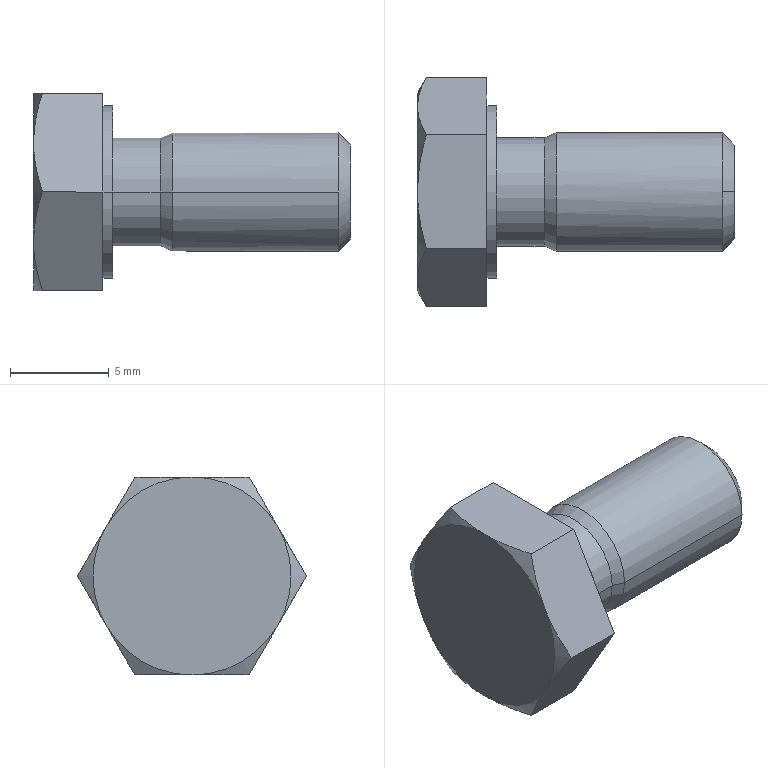Part | SolidWorks | features BaseBody 1 | 1 solid | 26 faces | box 16 x 11.547 x 10 mm | volume 654.588 mm3 | cone 10 | plane 10 | cylinder 6 | commonest cylinder face diameters 5.459 x2 6 x2 8.7 x2
STEP:
#1=CARTESIAN_POINT('',(3.,3.,0.));
#2=VERTEX_POINT('',#1);
#3=CARTESIAN_POINT('',(3.,-3.,0.));
#4=VERTEX_POINT('',#3);
#5=CARTESIAN_POINT('',(3.,0.,0.));
#6=DIRECTION('',(1.,0.,0.));
#7=DIRECTION('',(0.,1.,0.));
#8=AXIS2_PLACEMENT_3D('',#5,#6,#7);
#9=CIRCLE('',#8,3.);
#10=EDGE_CURVE('',#2,#4,#9,.T.);
#11=ORIENTED_EDGE('',*,*,#10,.T.);
#12=CARTESIAN_POINT('',(11.386,-3.,0.));
#13=VERTEX_POINT('',#12);
#14=CARTESIAN_POINT('',(7.5,-3.,0.));
#15=DIRECTION('',(1.,0.,0.));
#16=VECTOR('',#15,1000.);
#17=LINE('',#14,#16);
#18=EDGE_CURVE('',#4,#13,#17,.T.);
#19=ORIENTED_EDGE('',*,*,#18,.T.);
#20=CARTESIAN_POINT('',(11.386,0.,3.));
#21=VERTEX_POINT('',#20);
#22=CARTESIAN_POINT('',(11.386,0.,0.));
#23=DIRECTION('',(-1.,0.,0.));
#24=DIRECTION('',(0.,1.,0.));
#25=AXIS2_PLACEMENT_3D('',#22,#23,#24);
#26=CIRCLE('',#25,3.);
#27=EDGE_CURVE('',#13,#21,#26,.T.);
#28=ORIENTED_EDGE('',*,*,#27,.T.);
#29=CARTESIAN_POINT('',(11.386,3.,0.));
#30=VERTEX_POINT('',#29);
#31=CARTESIAN_POINT('',(11.386,0.,0.));
#32=DIRECTION('',(-1.,0.,0.));
#33=DIRECTION('',(0.,1.,0.));
#34=AXIS2_PLACEMENT_3D('',#31,#32,#33);
#35=CIRCLE('',#34,3.);
#36=EDGE_CURVE('',#21,#30,#35,.T.);
#37=ORIENTED_EDGE('',*,*,#36,.T.);
#38=CARTESIAN_POINT('',(7.5,3.,0.));
#39=DIRECTION('',(1.,0.,0.));
#40=VECTOR('',#39,1000.);
#41=LINE('',#38,#40);
#42=EDGE_CURVE('',#2,#30,#41,.T.);
#43=ORIENTED_EDGE('',*,*,#42,.F.);
#44=EDGE_LOOP('',(#11,#19,#28,#37,#43));
#45=FACE_OUTER_BOUND('',#44,.T.);
#46=CARTESIAN_POINT('',(7.5,0.,0.));
#47=DIRECTION('',(1.,0.,0.));
#48=DIRECTION('',(0.,1.,0.));
#49=AXIS2_PLACEMENT_3D('',#46,#47,#48);
#50=CYLINDRICAL_SURFACE('',#49,3.);
#51=ADVANCED_FACE('',(#45),#50,.T.);
#52=CARTESIAN_POINT('',(12.,0.,2.387));
#53=VERTEX_POINT('',#52);
#54=CARTESIAN_POINT('',(12.,0.,-2.387));
#55=VERTEX_POINT('',#54);
#56=CARTESIAN_POINT('',(12.,0.,0.));
#57=DIRECTION('',(-1.,0.,0.));
#58=DIRECTION('',(0.,0.,1.));
#59=AXIS2_PLACEMENT_3D('',#56,#57,#58);
#60=CIRCLE('',#59,2.387);
#61=EDGE_CURVE('',#53,#55,#60,.T.);
#62=ORIENTED_EDGE('',*,*,#61,.T.);
#63=CARTESIAN_POINT('',(11.386,0.,-3.));
#64=VERTEX_POINT('',#63);
#65=CARTESIAN_POINT('',(11.386,0.,-3.));
#66=DIRECTION('',(-0.7072,0.,-0.707));
#67=VECTOR('',#66,1000.);
#68=LINE('',#65,#67);
#69=EDGE_CURVE('',#55,#64,#68,.T.);
#70=ORIENTED_EDGE('',*,*,#69,.T.);
#71=CARTESIAN_POINT('',(11.386,0.,0.));
#72=DIRECTION('',(-1.,0.,0.));
#73=DIRECTION('',(0.,1.,0.));
#74=AXIS2_PLACEMENT_3D('',#71,#72,#73);
#75=CIRCLE('',#74,3.);
#76=EDGE_CURVE('',#30,#64,#75,.T.);
#77=ORIENTED_EDGE('',*,*,#76,.F.);
#78=ORIENTED_EDGE('',*,*,#36,.F.);
#79=CARTESIAN_POINT('',(11.386,0.,3.));
#80=DIRECTION('',(-0.7072,0.,0.707));
#81=VECTOR('',#80,1000.);
#82=LINE('',#79,#81);
#83=EDGE_CURVE('',#53,#21,#82,.T.);
#84=ORIENTED_EDGE('',*,*,#83,.F.);
#85=EDGE_LOOP('',(#62,#70,#77,#78,#84));
#86=FACE_OUTER_BOUND('',#85,.T.);
#87=CARTESIAN_POINT('',(11.386,0.,0.));
#88=DIRECTION('',(-1.,0.,0.));
#89=DIRECTION('',(0.,0.,1.));
#90=AXIS2_PLACEMENT_3D('',#87,#88,#89);
#91=CONICAL_SURFACE('',#90,3.,0.7853);
#92=ADVANCED_FACE('',(#86),#91,.T.);
#93=CARTESIAN_POINT('',(2.386,2.729,0.));
#94=VERTEX_POINT('',#93);
#95=CARTESIAN_POINT('',(2.386,-2.729,0.));
#96=VERTEX_POINT('',#95);
#97=CARTESIAN_POINT('',(2.386,0.,0.));
#98=DIRECTION('',(1.,0.,0.));
#99=DIRECTION('',(0.,1.,0.));
#100=AXIS2_PLACEMENT_3D('',#97,#98,#99);
#101=CIRCLE('',#100,2.729);
#102=EDGE_CURVE('',#94,#96,#101,.T.);
#103=ORIENTED_EDGE('',*,*,#102,.T.);
#104=CARTESIAN_POINT('',(3.,-3.,0.));
#105=DIRECTION('',(0.9149,-0.4036,0.));
#106=VECTOR('',#105,1000.);
#107=LINE('',#104,#106);
#108=EDGE_CURVE('',#96,#4,#107,.T.);
#109=ORIENTED_EDGE('',*,*,#108,.T.);
#110=ORIENTED_EDGE('',*,*,#10,.F.);
#111=CARTESIAN_POINT('',(3.,3.,0.));
#112=DIRECTION('',(0.9149,0.4036,0.));
#113=VECTOR('',#112,1000.);
#114=LINE('',#111,#113);
#115=EDGE_CURVE('',#94,#2,#114,.T.);
#116=ORIENTED_EDGE('',*,*,#115,.F.);
#117=EDGE_LOOP('',(#103,#109,#110,#116));
#118=FACE_OUTER_BOUND('',#117,.T.);
#119=CARTESIAN_POINT('',(3.,0.,0.));
#120=DIRECTION('',(1.,0.,0.));
#121=DIRECTION('',(0.,1.,0.));
#122=AXIS2_PLACEMENT_3D('',#119,#120,#121);
#123=CONICAL_SURFACE('',#122,3.,0.4154);
#124=ADVANCED_FACE('',(#118),#123,.T.);
#125=CARTESIAN_POINT('',(0.,2.729,0.));
#126=VERTEX_POINT('',#125);
#127=CARTESIAN_POINT('',(0.,-2.729,0.));
#128=VERTEX_POINT('',#127);
#129=CARTESIAN_POINT('',(0.,0.,0.));
#130=DIRECTION('',(1.,0.,0.));
#131=DIRECTION('',(0.,1.,0.));
#132=AXIS2_PLACEMENT_3D('',#129,#130,#131);
#133=CIRCLE('',#132,2.729);
#134=EDGE_CURVE('',#126,#128,#133,.T.);
#135=ORIENTED_EDGE('',*,*,#134,.T.);
#136=CARTESIAN_POINT('',(1.193,-2.729,0.));
#137=DIRECTION('',(1.,0.,0.));
#138=VECTOR('',#137,1000.);
#139=LINE('',#136,#138);
#140=EDGE_CURVE('',#128,#96,#139,.T.);
#141=ORIENTED_EDGE('',*,*,#140,.T.);
#142=ORIENTED_EDGE('',*,*,#102,.F.);
#143=CARTESIAN_POINT('',(1.193,2.729,0.));
#144=DIRECTION('',(1.,0.,0.));
#145=VECTOR('',#144,1000.);
#146=LINE('',#143,#145);
#147=EDGE_CURVE('',#126,#94,#146,.T.);
#148=ORIENTED_EDGE('',*,*,#147,.F.);
#149=EDGE_LOOP('',(#135,#141,#142,#148));
#150=FACE_OUTER_BOUND('',#149,.T.);
#151=CARTESIAN_POINT('',(1.193,0.,0.));
#152=DIRECTION('',(1.,0.,0.));
#153=DIRECTION('',(0.,1.,0.));
#154=AXIS2_PLACEMENT_3D('',#151,#152,#153);
#155=CYLINDRICAL_SURFACE('',#154,2.729);
#156=ADVANCED_FACE('',(#150),#155,.T.);
#157=CARTESIAN_POINT('',(-0.5001,4.35,0.));
#158=VERTEX_POINT('',#157);
#159=CARTESIAN_POINT('',(-0.5001,-4.35,0.));
#160=VERTEX_POINT('',#159);
#161=CARTESIAN_POINT('',(-0.5001,0.,0.));
#162=DIRECTION('',(1.,0.,0.));
#163=DIRECTION('',(0.,1.,0.));
#164=AXIS2_PLACEMENT_3D('',#161,#162,#163);
#165=CIRCLE('',#164,4.35);
#166=EDGE_CURVE('',#158,#160,#165,.T.);
#167=ORIENTED_EDGE('',*,*,#166,.T.);
#168=CARTESIAN_POINT('',(0.,-4.35,0.));
#169=VERTEX_POINT('',#168);
#170=CARTESIAN_POINT('',(-0.25,-4.35,0.));
#171=DIRECTION('',(1.,0.,0.));
#172=VECTOR('',#171,1000.);
#173=LINE('',#170,#172);
#174=EDGE_CURVE('',#160,#169,#173,.T.);
#175=ORIENTED_EDGE('',*,*,#174,.T.);
#176=CARTESIAN_POINT('',(0.,4.35,0.));
#177=VERTEX_POINT('',#176);
#178=CARTESIAN_POINT('',(0.,0.,0.));
#179=DIRECTION('',(1.,0.,0.));
#180=DIRECTION('',(0.,1.,0.));
#181=AXIS2_PLACEMENT_3D('',#178,#179,#180);
#182=CIRCLE('',#181,4.35);
#183=EDGE_CURVE('',#177,#169,#182,.T.);
#184=ORIENTED_EDGE('',*,*,#183,.F.);
#185=CARTESIAN_POINT('',(-0.25,4.35,0.));
#186=DIRECTION('',(1.,0.,0.));
#187=VECTOR('',#186,1000.);
#188=LINE('',#185,#187);
#189=EDGE_CURVE('',#158,#177,#188,.T.);
#190=ORIENTED_EDGE('',*,*,#189,.F.);
#191=EDGE_LOOP('',(#167,#175,#184,#190));
#192=FACE_OUTER_BOUND('',#191,.T.);
#193=CARTESIAN_POINT('',(-0.25,0.,0.));
#194=DIRECTION('',(1.,0.,0.));
#195=DIRECTION('',(0.,1.,0.));
#196=AXIS2_PLACEMENT_3D('',#193,#194,#195);
#197=CYLINDRICAL_SURFACE('',#196,4.35);
#198=ADVANCED_FACE('',(#192),#197,.T.);
#199=ORIENTED_EDGE('',*,*,#18,.F.);
#200=CARTESIAN_POINT('',(3.,0.,0.));
#201=DIRECTION('',(1.,0.,0.));
#202=DIRECTION('',(0.,1.,0.));
#203=AXIS2_PLACEMENT_3D('',#200,#201,#202);
#204=CIRCLE('',#203,3.);
#205=EDGE_CURVE('',#4,#2,#204,.T.);
#206=ORIENTED_EDGE('',*,*,#205,.T.);
#207=ORIENTED_EDGE('',*,*,#42,.T.);
#208=ORIENTED_EDGE('',*,*,#76,.T.);
#209=CARTESIAN_POINT('',(11.386,0.,0.));
#210=DIRECTION('',(-1.,0.,0.));
#211=DIRECTION('',(0.,1.,0.));
#212=AXIS2_PLACEMENT_3D('',#209,#210,#211);
#213=CIRCLE('',#212,3.);
#214=EDGE_CURVE('',#64,#13,#213,.T.);
#215=ORIENTED_EDGE('',*,*,#214,.T.);
#216=EDGE_LOOP('',(#199,#206,#207,#208,#215));
#217=FACE_OUTER_BOUND('',#216,.T.);
#218=CARTESIAN_POINT('',(7.5,0.,0.));
#219=DIRECTION('',(1.,0.,0.));
#220=DIRECTION('',(0.,1.,0.));
#221=AXIS2_PLACEMENT_3D('',#218,#219,#220);
#222=CYLINDRICAL_SURFACE('',#221,3.);
#223=ADVANCED_FACE('',(#217),#222,.T.);
#224=ORIENTED_EDGE('',*,*,#69,.F.);
#225=CARTESIAN_POINT('',(12.,0.,0.));
#226=DIRECTION('',(-1.,0.,0.));
#227=DIRECTION('',(0.,0.,1.));
#228=AXIS2_PLACEMENT_3D('',#225,#226,#227);
#229=CIRCLE('',#228,2.387);
#230=EDGE_CURVE('',#55,#53,#229,.T.);
#231=ORIENTED_EDGE('',*,*,#230,.T.);
#232=ORIENTED_EDGE('',*,*,#83,.T.);
#233=ORIENTED_EDGE('',*,*,#27,.F.);
#234=ORIENTED_EDGE('',*,*,#214,.F.);
#235=EDGE_LOOP('',(#224,#231,#232,#233,#234));
#236=FACE_OUTER_BOUND('',#235,.T.);
#237=CARTESIAN_POINT('',(11.386,0.,0.));
#238=DIRECTION('',(-1.,0.,0.));
#239=DIRECTION('',(0.,0.,1.));
#240=AXIS2_PLACEMENT_3D('',#237,#238,#239);
#241=CONICAL_SURFACE('',#240,3.,0.7853);
#242=ADVANCED_FACE('',(#236),#241,.T.);
#243=ORIENTED_EDGE('',*,*,#108,.F.);
#244=CARTESIAN_POINT('',(2.386,0.,0.));
#245=DIRECTION('',(1.,0.,0.));
#246=DIRECTION('',(0.,1.,0.));
#247=AXIS2_PLACEMENT_3D('',#244,#245,#246);
#248=CIRCLE('',#247,2.729);
#249=EDGE_CURVE('',#96,#94,#248,.T.);
#250=ORIENTED_EDGE('',*,*,#249,.T.);
#251=ORIENTED_EDGE('',*,*,#115,.T.);
#252=ORIENTED_EDGE('',*,*,#205,.F.);
#253=EDGE_LOOP('',(#243,#250,#251,#252));
#254=FACE_OUTER_BOUND('',#253,.T.);
#255=CARTESIAN_POINT('',(3.,0.,0.));
#256=DIRECTION('',(1.,0.,0.));
#257=DIRECTION('',(0.,1.,0.));
#258=AXIS2_PLACEMENT_3D('',#255,#256,#257);
#259=CONICAL_SURFACE('',#258,3.,0.4154);
#260=ADVANCED_FACE('',(#254),#259,.T.);
#261=ORIENTED_EDGE('',*,*,#61,.F.);
#262=ORIENTED_EDGE('',*,*,#230,.F.);
#263=EDGE_LOOP('',(#261,#262));
#264=FACE_OUTER_BOUND('',#263,.T.);
#265=CARTESIAN_POINT('',(12.,1.5,0.));
#266=DIRECTION('',(1.,0.,0.));
#267=DIRECTION('',(0.,1.,0.));
#268=AXIS2_PLACEMENT_3D('',#265,#266,#267);
#269=PLANE('',#268);
#270=ADVANCED_FACE('',(#264),#269,.T.);
#271=ORIENTED_EDGE('',*,*,#140,.F.);
#272=CARTESIAN_POINT('',(0.,0.,0.));
#273=DIRECTION('',(1.,0.,0.));
#274=DIRECTION('',(0.,1.,0.));
#275=AXIS2_PLACEMENT_3D('',#272,#273,#274);
#276=CIRCLE('',#275,2.729);
#277=EDGE_CURVE('',#128,#126,#276,.T.);
#278=ORIENTED_EDGE('',*,*,#277,.T.);
#279=ORIENTED_EDGE('',*,*,#147,.T.);
#280=ORIENTED_EDGE('',*,*,#249,.F.);
#281=EDGE_LOOP('',(#271,#278,#279,#280));
#282=FACE_OUTER_BOUND('',#281,.T.);
#283=CARTESIAN_POINT('',(1.193,0.,0.));
#284=DIRECTION('',(1.,0.,0.));
#285=DIRECTION('',(0.,1.,0.));
#286=AXIS2_PLACEMENT_3D('',#283,#284,#285);
#287=CYLINDRICAL_SURFACE('',#286,2.729);
#288=ADVANCED_FACE('',(#282),#287,.T.);
#289=ORIENTED_EDGE('',*,*,#134,.F.);
#290=ORIENTED_EDGE('',*,*,#277,.F.);
#291=EDGE_LOOP('',(#289,#290));
#292=FACE_BOUND('',#291,.T.);
#293=ORIENTED_EDGE('',*,*,#183,.T.);
#294=CARTESIAN_POINT('',(0.,0.,0.));
#295=DIRECTION('',(1.,0.,0.));
#296=DIRECTION('',(0.,1.,0.));
#297=AXIS2_PLACEMENT_3D('',#294,#295,#296);
#298=CIRCLE('',#297,4.35);
#299=EDGE_CURVE('',#169,#177,#298,.T.);
#300=ORIENTED_EDGE('',*,*,#299,.T.);
#301=EDGE_LOOP('',(#293,#300));
#302=FACE_OUTER_BOUND('',#301,.T.);
#303=CARTESIAN_POINT('',(0.,3.54,0.));
#304=DIRECTION('',(1.,0.,0.));
#305=DIRECTION('',(0.,1.,0.));
#306=AXIS2_PLACEMENT_3D('',#303,#304,#305);
#307=PLANE('',#306);
#308=ADVANCED_FACE('',(#292,#302),#307,.T.);
#309=ORIENTED_EDGE('',*,*,#174,.F.);
#310=CARTESIAN_POINT('',(-0.5001,0.,0.));
#311=DIRECTION('',(1.,0.,0.));
#312=DIRECTION('',(0.,1.,0.));
#313=AXIS2_PLACEMENT_3D('',#310,#311,#312);
#314=CIRCLE('',#313,4.35);
#315=EDGE_CURVE('',#160,#158,#314,.T.);
#316=ORIENTED_EDGE('',*,*,#315,.T.);
#317=ORIENTED_EDGE('',*,*,#189,.T.);
#318=ORIENTED_EDGE('',*,*,#299,.F.);
#319=EDGE_LOOP('',(#309,#316,#317,#318));
#320=FACE_OUTER_BOUND('',#319,.T.);
#321=CARTESIAN_POINT('',(-0.25,0.,0.));
#322=DIRECTION('',(1.,0.,0.));
#323=DIRECTION('',(0.,1.,0.));
#324=AXIS2_PLACEMENT_3D('',#321,#322,#323);
#325=CYLINDRICAL_SURFACE('',#324,4.35);
#326=ADVANCED_FACE('',(#320),#325,.T.);
#327=ORIENTED_EDGE('',*,*,#166,.F.);
#328=ORIENTED_EDGE('',*,*,#315,.F.);
#329=EDGE_LOOP('',(#327,#328));
#330=FACE_BOUND('',#329,.T.);
#331=CARTESIAN_POINT('',(-0.5001,-2.887,-5.));
#332=VERTEX_POINT('',#331);
#333=CARTESIAN_POINT('',(-0.5001,2.887,-5.));
#334=VERTEX_POINT('',#333);
#335=CARTESIAN_POINT('',(-0.5001,0.,-5.));
#336=DIRECTION('',(0.,1.,0.));
#337=VECTOR('',#336,1000.);
#338=LINE('',#335,#337);
#339=EDGE_CURVE('',#332,#334,#338,.T.);
#340=ORIENTED_EDGE('',*,*,#339,.T.);
#341=CARTESIAN_POINT('',(-0.5001,5.774,0.));
#342=VERTEX_POINT('',#341);
#343=CARTESIAN_POINT('',(-0.5001,2.887,-5.));
#344=DIRECTION('',(0.,0.5,0.866));
#345=VECTOR('',#344,1000.);
#346=LINE('',#343,#345);
#347=EDGE_CURVE('',#334,#342,#346,.T.);
#348=ORIENTED_EDGE('',*,*,#347,.T.);
#349=CARTESIAN_POINT('',(-0.5001,2.887,5.));
#350=VERTEX_POINT('',#349);
#351=CARTESIAN_POINT('',(-0.5001,5.774,0.));
#352=DIRECTION('',(0.,-0.5,0.866));
#353=VECTOR('',#352,1000.);
#354=LINE('',#351,#353);
#355=EDGE_CURVE('',#342,#350,#354,.T.);
#356=ORIENTED_EDGE('',*,*,#355,.T.);
#357=CARTESIAN_POINT('',(-0.5001,-2.887,5.));
#358=VERTEX_POINT('',#357);
#359=CARTESIAN_POINT('',(-0.5001,0.,5.));
#360=DIRECTION('',(0.,-1.,0.));
#361=VECTOR('',#360,1000.);
#362=LINE('',#359,#361);
#363=EDGE_CURVE('',#350,#358,#362,.T.);
#364=ORIENTED_EDGE('',*,*,#363,.T.);
#365=CARTESIAN_POINT('',(-0.5001,-5.774,0.));
#366=VERTEX_POINT('',#365);
#367=CARTESIAN_POINT('',(-0.5001,-2.887,5.));
#368=DIRECTION('',(0.,-0.5,-0.866));
#369=VECTOR('',#368,1000.);
#370=LINE('',#367,#369);
#371=EDGE_CURVE('',#358,#366,#370,.T.);
#372=ORIENTED_EDGE('',*,*,#371,.T.);
#373=CARTESIAN_POINT('',(-0.5001,-5.774,0.));
#374=DIRECTION('',(0.,0.5,-0.866));
#375=VECTOR('',#374,1000.);
#376=LINE('',#373,#375);
#377=EDGE_CURVE('',#366,#332,#376,.T.);
#378=ORIENTED_EDGE('',*,*,#377,.T.);
#379=EDGE_LOOP('',(#340,#348,#356,#364,#372,#378));
#380=FACE_OUTER_BOUND('',#379,.T.);
#381=CARTESIAN_POINT('',(-0.5001,0.,0.));
#382=DIRECTION('',(1.,0.,0.));
#383=DIRECTION('',(0.,1.,0.));
#384=AXIS2_PLACEMENT_3D('',#381,#382,#383);
#385=PLANE('',#384);
#386=ADVANCED_FACE('',(#330,#380),#385,.T.);
#387=ORIENTED_EDGE('',*,*,#347,.F.);
#388=CARTESIAN_POINT('',(-3.554,2.887,-5.));
#389=VERTEX_POINT('',#388);
#390=CARTESIAN_POINT('',(-0.5001,2.887,-5.));
#391=DIRECTION('',(-1.,0.,0.));
#392=VECTOR('',#391,1000.);
#393=LINE('',#390,#392);
#394=EDGE_CURVE('',#334,#389,#393,.T.);
#395=ORIENTED_EDGE('',*,*,#394,.T.);
#396=CARTESIAN_POINT('',(-4.,4.33,-2.5));
#397=VERTEX_POINT('',#396);
#398=CARTESIAN_POINT('',(-3.554,2.887,-5.));
#399=CARTESIAN_POINT('',(-3.826,3.358,-4.183));
#400=CARTESIAN_POINT('',(-4.,3.837,-3.353));
#401=CARTESIAN_POINT('',(-4.,4.33,-2.5));
#402=B_SPLINE_CURVE_WITH_KNOTS('',3,(#398,#399,#400,#401),.UNSPECIFIED.,.F.,.F.,(4,4),(0.,0.002921),.UNSPECIFIED.);
#403=EDGE_CURVE('',#389,#397,#402,.T.);
#404=ORIENTED_EDGE('',*,*,#403,.T.);
#405=CARTESIAN_POINT('',(-3.554,5.774,0.));
#406=VERTEX_POINT('',#405);
#407=CARTESIAN_POINT('',(-4.,4.33,-2.5));
#408=CARTESIAN_POINT('',(-4.,4.823,-1.647));
#409=CARTESIAN_POINT('',(-3.826,5.302,-0.8168));
#410=CARTESIAN_POINT('',(-3.554,5.774,0.));
#411=B_SPLINE_CURVE_WITH_KNOTS('',3,(#407,#408,#409,#410),.UNSPECIFIED.,.F.,.F.,(4,4),(0.,0.002921),.UNSPECIFIED.);
#412=EDGE_CURVE('',#397,#406,#411,.T.);
#413=ORIENTED_EDGE('',*,*,#412,.T.);
#414=CARTESIAN_POINT('',(-0.5001,5.774,0.));
#415=DIRECTION('',(1.,0.,0.));
#416=VECTOR('',#415,1000.);
#417=LINE('',#414,#416);
#418=EDGE_CURVE('',#406,#342,#417,.T.);
#419=ORIENTED_EDGE('',*,*,#418,.T.);
#420=EDGE_LOOP('',(#387,#395,#404,#413,#419));
#421=FACE_OUTER_BOUND('',#420,.T.);
#422=CARTESIAN_POINT('',(-0.5001,2.887,-5.));
#423=DIRECTION('',(0.,0.866,-0.5));
#424=DIRECTION('',(0.,0.5,0.866));
#425=AXIS2_PLACEMENT_3D('',#422,#423,#424);
#426=PLANE('',#425);
#427=ADVANCED_FACE('',(#421),#426,.T.);
#428=ORIENTED_EDGE('',*,*,#339,.F.);
#429=CARTESIAN_POINT('',(-3.554,-2.887,-5.));
#430=VERTEX_POINT('',#429);
#431=CARTESIAN_POINT('',(-0.5001,-2.887,-5.));
#432=DIRECTION('',(-1.,0.,0.));
#433=VECTOR('',#432,1000.);
#434=LINE('',#431,#433);
#435=EDGE_CURVE('',#332,#430,#434,.T.);
#436=ORIENTED_EDGE('',*,*,#435,.T.);
#437=CARTESIAN_POINT('',(-4.,0.,-5.));
#438=VERTEX_POINT('',#437);
#439=CARTESIAN_POINT('',(-3.554,-2.887,-5.));
#440=CARTESIAN_POINT('',(-3.826,-1.944,-5.));
#441=CARTESIAN_POINT('',(-4.,-0.9853,-5.));
#442=CARTESIAN_POINT('',(-4.,0.,-5.));
#443=B_SPLINE_CURVE_WITH_KNOTS('',3,(#439,#440,#441,#442),.UNSPECIFIED.,.F.,.F.,(4,4),(0.,0.002921),.UNSPECIFIED.);
#444=EDGE_CURVE('',#430,#438,#443,.T.);
#445=ORIENTED_EDGE('',*,*,#444,.T.);
#446=CARTESIAN_POINT('',(-4.,0.,-5.));
#447=CARTESIAN_POINT('',(-4.,0.9853,-5.));
#448=CARTESIAN_POINT('',(-3.826,1.944,-5.));
#449=CARTESIAN_POINT('',(-3.554,2.887,-5.));
#450=B_SPLINE_CURVE_WITH_KNOTS('',3,(#446,#447,#448,#449),.UNSPECIFIED.,.F.,.F.,(4,4),(0.,0.002921),.UNSPECIFIED.);
#451=EDGE_CURVE('',#438,#389,#450,.T.);
#452=ORIENTED_EDGE('',*,*,#451,.T.);
#453=ORIENTED_EDGE('',*,*,#394,.F.);
#454=EDGE_LOOP('',(#428,#436,#445,#452,#453));
#455=FACE_OUTER_BOUND('',#454,.T.);
#456=CARTESIAN_POINT('',(-0.5001,-2.887,-5.));
#457=DIRECTION('',(0.,0.,-1.));
#458=DIRECTION('',(0.,1.,0.));
#459=AXIS2_PLACEMENT_3D('',#456,#457,#458);
#460=PLANE('',#459);
#461=ADVANCED_FACE('',(#455),#460,.T.);
#462=CARTESIAN_POINT('',(-3.554,-5.774,0.));
#463=VERTEX_POINT('',#462);
#464=CARTESIAN_POINT('',(-0.5001,-5.774,0.));
#465=DIRECTION('',(-1.,0.,0.));
#466=VECTOR('',#465,1000.);
#467=LINE('',#464,#466);
#468=EDGE_CURVE('',#366,#463,#467,.T.);
#469=ORIENTED_EDGE('',*,*,#468,.T.);
#470=CARTESIAN_POINT('',(-4.,-4.33,-2.5));
#471=VERTEX_POINT('',#470);
#472=CARTESIAN_POINT('',(-3.554,-5.774,0.));
#473=CARTESIAN_POINT('',(-3.826,-5.302,-0.8168));
#474=CARTESIAN_POINT('',(-4.,-4.823,-1.647));
#475=CARTESIAN_POINT('',(-4.,-4.33,-2.5));
#476=B_SPLINE_CURVE_WITH_KNOTS('',3,(#472,#473,#474,#475),.UNSPECIFIED.,.F.,.F.,(4,4),(0.,0.002921),.UNSPECIFIED.);
#477=EDGE_CURVE('',#463,#471,#476,.T.);
#478=ORIENTED_EDGE('',*,*,#477,.T.);
#479=CARTESIAN_POINT('',(-4.,-4.33,-2.5));
#480=CARTESIAN_POINT('',(-4.,-3.837,-3.353));
#481=CARTESIAN_POINT('',(-3.826,-3.358,-4.183));
#482=CARTESIAN_POINT('',(-3.554,-2.887,-5.));
#483=B_SPLINE_CURVE_WITH_KNOTS('',3,(#479,#480,#481,#482),.UNSPECIFIED.,.F.,.F.,(4,4),(0.,0.002921),.UNSPECIFIED.);
#484=EDGE_CURVE('',#471,#430,#483,.T.);
#485=ORIENTED_EDGE('',*,*,#484,.T.);
#486=ORIENTED_EDGE('',*,*,#435,.F.);
#487=ORIENTED_EDGE('',*,*,#377,.F.);
#488=EDGE_LOOP('',(#469,#478,#485,#486,#487));
#489=FACE_OUTER_BOUND('',#488,.T.);
#490=CARTESIAN_POINT('',(-0.5001,-5.774,0.));
#491=DIRECTION('',(0.,-0.866,-0.5));
#492=DIRECTION('',(0.,0.5,-0.866));
#493=AXIS2_PLACEMENT_3D('',#490,#491,#492);
#494=PLANE('',#493);
#495=ADVANCED_FACE('',(#489),#494,.T.);
#496=CARTESIAN_POINT('',(-3.554,-2.887,5.));
#497=VERTEX_POINT('',#496);
#498=CARTESIAN_POINT('',(-0.5001,-2.887,5.));
#499=DIRECTION('',(-1.,0.,0.));
#500=VECTOR('',#499,1000.);
#501=LINE('',#498,#500);
#502=EDGE_CURVE('',#358,#497,#501,.T.);
#503=ORIENTED_EDGE('',*,*,#502,.T.);
#504=CARTESIAN_POINT('',(-4.,-4.33,2.5));
#505=VERTEX_POINT('',#504);
#506=CARTESIAN_POINT('',(-3.554,-2.887,5.));
#507=CARTESIAN_POINT('',(-3.826,-3.358,4.183));
#508=CARTESIAN_POINT('',(-4.,-3.837,3.353));
#509=CARTESIAN_POINT('',(-4.,-4.33,2.5));
#510=B_SPLINE_CURVE_WITH_KNOTS('',3,(#506,#507,#508,#509),.UNSPECIFIED.,.F.,.F.,(4,4),(0.,0.002921),.UNSPECIFIED.);
#511=EDGE_CURVE('',#497,#505,#510,.T.);
#512=ORIENTED_EDGE('',*,*,#511,.T.);
#513=CARTESIAN_POINT('',(-4.,-4.33,2.5));
#514=CARTESIAN_POINT('',(-4.,-4.823,1.647));
#515=CARTESIAN_POINT('',(-3.826,-5.302,0.8168));
#516=CARTESIAN_POINT('',(-3.554,-5.774,0.));
#517=B_SPLINE_CURVE_WITH_KNOTS('',3,(#513,#514,#515,#516),.UNSPECIFIED.,.F.,.F.,(4,4),(0.,0.002921),.UNSPECIFIED.);
#518=EDGE_CURVE('',#505,#463,#517,.T.);
#519=ORIENTED_EDGE('',*,*,#518,.T.);
#520=ORIENTED_EDGE('',*,*,#468,.F.);
#521=ORIENTED_EDGE('',*,*,#371,.F.);
#522=EDGE_LOOP('',(#503,#512,#519,#520,#521));
#523=FACE_OUTER_BOUND('',#522,.T.);
#524=CARTESIAN_POINT('',(-0.5001,-2.887,5.));
#525=DIRECTION('',(0.,-0.866,0.5));
#526=DIRECTION('',(0.,-0.5,-0.866));
#527=AXIS2_PLACEMENT_3D('',#524,#525,#526);
#528=PLANE('',#527);
#529=ADVANCED_FACE('',(#523),#528,.T.);
#530=CARTESIAN_POINT('',(-3.554,2.887,5.));
#531=VERTEX_POINT('',#530);
#532=CARTESIAN_POINT('',(-0.5001,2.887,5.));
#533=DIRECTION('',(-1.,0.,0.));
#534=VECTOR('',#533,1000.);
#535=LINE('',#532,#534);
#536=EDGE_CURVE('',#350,#531,#535,.T.);
#537=ORIENTED_EDGE('',*,*,#536,.T.);
#538=CARTESIAN_POINT('',(-4.,0.,5.));
#539=VERTEX_POINT('',#538);
#540=CARTESIAN_POINT('',(-3.554,2.887,5.));
#541=CARTESIAN_POINT('',(-3.826,1.944,5.));
#542=CARTESIAN_POINT('',(-4.,0.9853,5.));
#543=CARTESIAN_POINT('',(-4.,0.,5.));
#544=B_SPLINE_CURVE_WITH_KNOTS('',3,(#540,#541,#542,#543),.UNSPECIFIED.,.F.,.F.,(4,4),(0.,0.002921),.UNSPECIFIED.);
#545=EDGE_CURVE('',#531,#539,#544,.T.);
#546=ORIENTED_EDGE('',*,*,#545,.T.);
#547=CARTESIAN_POINT('',(-4.,0.,5.));
#548=CARTESIAN_POINT('',(-4.,-0.9853,5.));
#549=CARTESIAN_POINT('',(-3.826,-1.944,5.));
#550=CARTESIAN_POINT('',(-3.554,-2.887,5.));
#551=B_SPLINE_CURVE_WITH_KNOTS('',3,(#547,#548,#549,#550),.UNSPECIFIED.,.F.,.F.,(4,4),(0.,0.002921),.UNSPECIFIED.);
#552=EDGE_CURVE('',#539,#497,#551,.T.);
#553=ORIENTED_EDGE('',*,*,#552,.T.);
#554=ORIENTED_EDGE('',*,*,#502,.F.);
#555=ORIENTED_EDGE('',*,*,#363,.F.);
#556=EDGE_LOOP('',(#537,#546,#553,#554,#555));
#557=FACE_OUTER_BOUND('',#556,.T.);
#558=CARTESIAN_POINT('',(-0.5001,2.887,5.));
#559=DIRECTION('',(0.,0.,1.));
#560=DIRECTION('',(0.,-1.,0.));
#561=AXIS2_PLACEMENT_3D('',#558,#559,#560);
#562=PLANE('',#561);
#563=ADVANCED_FACE('',(#557),#562,.T.);
#564=ORIENTED_EDGE('',*,*,#355,.F.);
#565=ORIENTED_EDGE('',*,*,#418,.F.);
#566=CARTESIAN_POINT('',(-4.,4.33,2.5));
#567=VERTEX_POINT('',#566);
#568=CARTESIAN_POINT('',(-3.554,5.774,0.));
#569=CARTESIAN_POINT('',(-3.826,5.302,0.8168));
#570=CARTESIAN_POINT('',(-4.,4.823,1.647));
#571=CARTESIAN_POINT('',(-4.,4.33,2.5));
#572=B_SPLINE_CURVE_WITH_KNOTS('',3,(#568,#569,#570,#571),.UNSPECIFIED.,.F.,.F.,(4,4),(0.,0.002921),.UNSPECIFIED.);
#573=EDGE_CURVE('',#406,#567,#572,.T.);
#574=ORIENTED_EDGE('',*,*,#573,.T.);
#575=CARTESIAN_POINT('',(-4.,4.33,2.5));
#576=CARTESIAN_POINT('',(-4.,3.837,3.353));
#577=CARTESIAN_POINT('',(-3.826,3.358,4.183));
#578=CARTESIAN_POINT('',(-3.554,2.887,5.));
#579=B_SPLINE_CURVE_WITH_KNOTS('',3,(#575,#576,#577,#578),.UNSPECIFIED.,.F.,.F.,(4,4),(0.,0.002921),.UNSPECIFIED.);
#580=EDGE_CURVE('',#567,#531,#579,.T.);
#581=ORIENTED_EDGE('',*,*,#580,.T.);
#582=ORIENTED_EDGE('',*,*,#536,.F.);
#583=EDGE_LOOP('',(#564,#565,#574,#581,#582));
#584=FACE_OUTER_BOUND('',#583,.T.);
#585=CARTESIAN_POINT('',(-0.5001,5.774,0.));
#586=DIRECTION('',(0.,0.866,0.5));
#587=DIRECTION('',(0.,-0.5,0.866));
#588=AXIS2_PLACEMENT_3D('',#585,#586,#587);
#589=PLANE('',#588);
#590=ADVANCED_FACE('',(#584),#589,.T.);
#591=CARTESIAN_POINT('',(-4.,0.,0.));
#592=DIRECTION('',(1.,0.,0.));
#593=DIRECTION('',(0.,0.,-1.));
#594=AXIS2_PLACEMENT_3D('',#591,#592,#593);
#595=CIRCLE('',#594,5.);
#596=EDGE_CURVE('',#397,#567,#595,.T.);
#597=ORIENTED_EDGE('',*,*,#596,.T.);
#598=ORIENTED_EDGE('',*,*,#573,.F.);
#599=ORIENTED_EDGE('',*,*,#412,.F.);
#600=EDGE_LOOP('',(#597,#598,#599));
#601=FACE_OUTER_BOUND('',#600,.T.);
#602=CARTESIAN_POINT('',(-3.551,0.,0.));
#603=DIRECTION('',(1.,0.,0.));
#604=DIRECTION('',(0.,0.,-1.));
#605=AXIS2_PLACEMENT_3D('',#602,#603,#604);
#606=CONICAL_SURFACE('',#605,5.778,1.047);
#607=ADVANCED_FACE('',(#601),#606,.T.);
#608=CARTESIAN_POINT('',(-4.,0.,0.));
#609=DIRECTION('',(1.,0.,0.));
#610=DIRECTION('',(0.,0.,-1.));
#611=AXIS2_PLACEMENT_3D('',#608,#609,#610);
#612=CIRCLE('',#611,5.);
#613=EDGE_CURVE('',#438,#397,#612,.T.);
#614=ORIENTED_EDGE('',*,*,#613,.T.);
#615=ORIENTED_EDGE('',*,*,#403,.F.);
#616=ORIENTED_EDGE('',*,*,#451,.F.);
#617=EDGE_LOOP('',(#614,#615,#616));
#618=FACE_OUTER_BOUND('',#617,.T.);
#619=CARTESIAN_POINT('',(-3.551,0.,0.));
#620=DIRECTION('',(1.,0.,0.));
#621=DIRECTION('',(0.,0.,-1.));
#622=AXIS2_PLACEMENT_3D('',#619,#620,#621);
#623=CONICAL_SURFACE('',#622,5.778,1.047);
#624=ADVANCED_FACE('',(#618),#623,.T.);
#625=ORIENTED_EDGE('',*,*,#484,.F.);
#626=CARTESIAN_POINT('',(-4.,0.,0.));
#627=DIRECTION('',(1.,0.,0.));
#628=DIRECTION('',(0.,0.,-1.));
#629=AXIS2_PLACEMENT_3D('',#626,#627,#628);
#630=CIRCLE('',#629,5.);
#631=EDGE_CURVE('',#471,#438,#630,.T.);
#632=ORIENTED_EDGE('',*,*,#631,.T.);
#633=ORIENTED_EDGE('',*,*,#444,.F.);
#634=EDGE_LOOP('',(#625,#632,#633));
#635=FACE_OUTER_BOUND('',#634,.T.);
#636=CARTESIAN_POINT('',(-3.551,0.,0.));
#637=DIRECTION('',(1.,0.,0.));
#638=DIRECTION('',(0.,0.,-1.));
#639=AXIS2_PLACEMENT_3D('',#636,#637,#638);
#640=CONICAL_SURFACE('',#639,5.778,1.047);
#641=ADVANCED_FACE('',(#635),#640,.T.);
#642=ORIENTED_EDGE('',*,*,#518,.F.);
#643=CARTESIAN_POINT('',(-4.,0.,0.));
#644=DIRECTION('',(1.,0.,0.));
#645=DIRECTION('',(0.,0.,-1.));
#646=AXIS2_PLACEMENT_3D('',#643,#644,#645);
#647=CIRCLE('',#646,5.);
#648=EDGE_CURVE('',#505,#471,#647,.T.);
#649=ORIENTED_EDGE('',*,*,#648,.T.);
#650=ORIENTED_EDGE('',*,*,#477,.F.);
#651=EDGE_LOOP('',(#642,#649,#650));
#652=FACE_OUTER_BOUND('',#651,.T.);
#653=CARTESIAN_POINT('',(-3.551,0.,0.));
#654=DIRECTION('',(1.,0.,0.));
#655=DIRECTION('',(0.,0.,-1.));
#656=AXIS2_PLACEMENT_3D('',#653,#654,#655);
#657=CONICAL_SURFACE('',#656,5.778,1.047);
#658=ADVANCED_FACE('',(#652),#657,.T.);
#659=ORIENTED_EDGE('',*,*,#552,.F.);
#660=CARTESIAN_POINT('',(-4.,0.,0.));
#661=DIRECTION('',(1.,0.,0.));
#662=DIRECTION('',(0.,0.,-1.));
#663=AXIS2_PLACEMENT_3D('',#660,#661,#662);
#664=CIRCLE('',#663,5.);
#665=EDGE_CURVE('',#539,#505,#664,.T.);
#666=ORIENTED_EDGE('',*,*,#665,.T.);
#667=ORIENTED_EDGE('',*,*,#511,.F.);
#668=EDGE_LOOP('',(#659,#666,#667));
#669=FACE_OUTER_BOUND('',#668,.T.);
#670=CARTESIAN_POINT('',(-3.551,0.,0.));
#671=DIRECTION('',(1.,0.,0.));
#672=DIRECTION('',(0.,0.,-1.));
#673=AXIS2_PLACEMENT_3D('',#670,#671,#672);
#674=CONICAL_SURFACE('',#673,5.778,1.047);
#675=ADVANCED_FACE('',(#669),#674,.T.);
#676=CARTESIAN_POINT('',(-4.,0.,0.));
#677=DIRECTION('',(1.,0.,0.));
#678=DIRECTION('',(0.,0.,-1.));
#679=AXIS2_PLACEMENT_3D('',#676,#677,#678);
#680=CIRCLE('',#679,5.);
#681=EDGE_CURVE('',#567,#539,#680,.T.);
#682=ORIENTED_EDGE('',*,*,#681,.T.);
#683=ORIENTED_EDGE('',*,*,#545,.F.);
#684=ORIENTED_EDGE('',*,*,#580,.F.);
#685=EDGE_LOOP('',(#682,#683,#684));
#686=FACE_OUTER_BOUND('',#685,.T.);
#687=CARTESIAN_POINT('',(-3.551,0.,0.));
#688=DIRECTION('',(1.,0.,0.));
#689=DIRECTION('',(0.,0.,-1.));
#690=AXIS2_PLACEMENT_3D('',#687,#688,#689);
#691=CONICAL_SURFACE('',#690,5.778,1.047);
#692=ADVANCED_FACE('',(#686),#691,.T.);
#693=ORIENTED_EDGE('',*,*,#596,.F.);
#694=ORIENTED_EDGE('',*,*,#613,.F.);
#695=ORIENTED_EDGE('',*,*,#631,.F.);
#696=ORIENTED_EDGE('',*,*,#648,.F.);
#697=ORIENTED_EDGE('',*,*,#665,.F.);
#698=ORIENTED_EDGE('',*,*,#681,.F.);
#699=EDGE_LOOP('',(#693,#694,#695,#696,#697,#698));
#700=FACE_OUTER_BOUND('',#699,.T.);
#701=CARTESIAN_POINT('',(-4.,0.,0.));
#702=DIRECTION('',(1.,0.,0.));
#703=DIRECTION('',(0.,1.,0.));
#704=AXIS2_PLACEMENT_3D('',#701,#702,#703);
#705=PLANE('',#704);
#706=ADVANCED_FACE('',(#700),#705,.F.);
#707=CLOSED_SHELL('',(#51,#92,#124,#156,#198,#223,#242,#260,#270,#288,#308,#326,#386,#427,#461,#495,#529,#563,#590,#607,#624,#641,#658,#675,#692,#706));
#708=MANIFOLD_SOLID_BREP('',#707);
#709=CARTESIAN_POINT('',(0.,0.,0.));
#710=DIRECTION('',(0.,0.,1.));
#711=DIRECTION('',(1.,0.,0.));
#712=AXIS2_PLACEMENT_3D('',#709,#710,#711);
#713=(LENGTH_UNIT()NAMED_UNIT(*)SI_UNIT(.MILLI.,.METRE.));
#714=UNCERTAINTY_MEASURE_WITH_UNIT(LENGTH_MEASURE(0.00001),#713,'','');
#715=(NAMED_UNIT(*)PLANE_ANGLE_UNIT()SI_UNIT($,.RADIAN.));
#716=(NAMED_UNIT(*)SI_UNIT($,.STERADIAN.)SOLID_ANGLE_UNIT());
#717=(GEOMETRIC_REPRESENTATION_CONTEXT(3)GLOBAL_UNCERTAINTY_ASSIGNED_CONTEXT((#714))GLOBAL_UNIT_ASSIGNED_CONTEXT((#713,#715,#716))REPRESENTATION_CONTEXT('',''));
#718=ADVANCED_BREP_SHAPE_REPRESENTATION('',(#708,#712),#717);